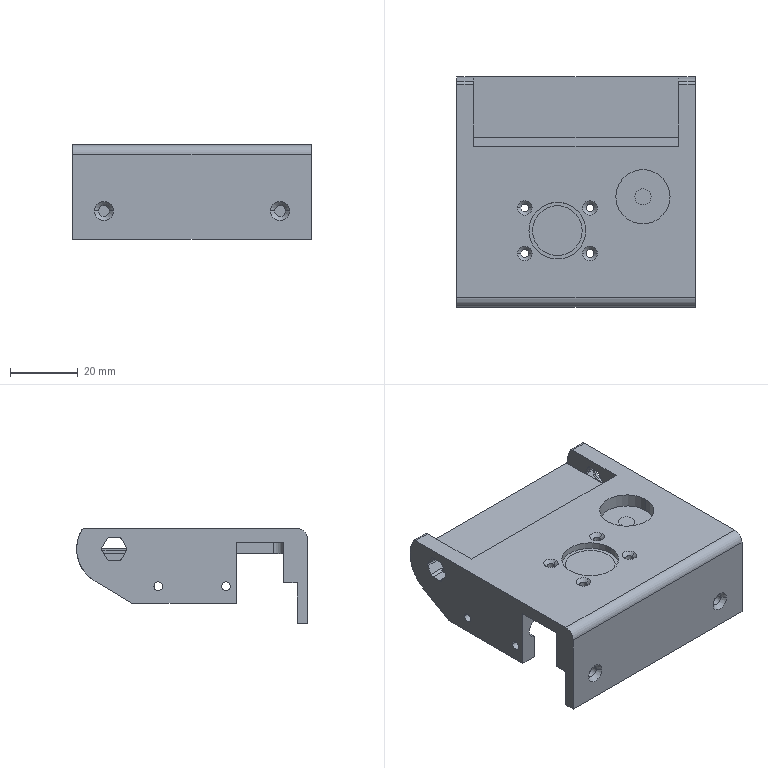Part | 5 solids | 145 faces | box 70.5 x 68.1 x 28 mm | volume 47697 mm3 | cylinder 67 | plane 56 | cone 20 | torus 2 | commonest cylinder face diameters 2 x16 2.3 x8 2.6 x7 6 x7 22.2 x5 1.6 x4